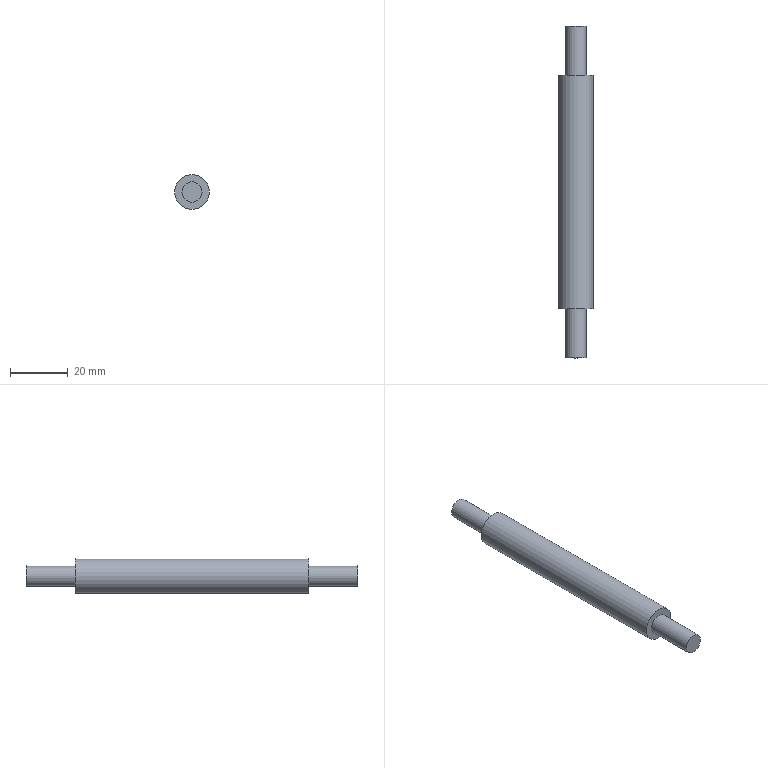Part | STEP file | 2-04.2 | 1 solid | 7 faces | box 12 x 115 x 12 mm | volume 10469 mm3 | plane 4 | cylinder 3 | commonest cylinder face diameters 7 x2 12 x1
STEP:
#1=CARTESIAN_POINT('',(0.,0.,0.));
#2=DIRECTION('',(0.,0.,1.));
#3=DIRECTION('',(1.,0.,0.));
#4=AXIS2_PLACEMENT_3D('',#1,#2,#3);
#5=CARTESIAN_POINT('',(6.,-40.5,0.));
#6=VERTEX_POINT('',#5);
#7=CARTESIAN_POINT('',(6.,40.5,0.));
#8=VERTEX_POINT('',#7);
#9=CARTESIAN_POINT('',(6.,-40.5,0.));
#10=DIRECTION('',(0.,1.,0.));
#11=VECTOR('',#10,1.);
#12=LINE('',#9,#11);
#13=CARTESIAN_POINT('',(0.,-40.5,0.));
#14=DIRECTION('',(0.,1.,0.));
#15=DIRECTION('',(1.,0.,0.));
#16=AXIS2_PLACEMENT_3D('',#13,#14,#15);
#17=CYLINDRICAL_SURFACE('',#16,6.);
#18=CARTESIAN_POINT('',(6.283,0.));
#19=DIRECTION('',(0.,1.));
#20=VECTOR('',#19,1.);
#21=LINE('',#18,#20);
#22=(GEOMETRIC_REPRESENTATION_CONTEXT(2)PARAMETRIC_REPRESENTATION_CONTEXT()REPRESENTATION_CONTEXT('',''));
#23=DEFINITIONAL_REPRESENTATION('',(#21),#22);
#24=PCURVE('',#17,#23);
#25=CARTESIAN_POINT('',(0.,0.));
#26=DIRECTION('',(0.,1.));
#27=VECTOR('',#26,1.);
#28=LINE('',#25,#27);
#29=(GEOMETRIC_REPRESENTATION_CONTEXT(2)PARAMETRIC_REPRESENTATION_CONTEXT()REPRESENTATION_CONTEXT('',''));
#30=DEFINITIONAL_REPRESENTATION('',(#28),#29);
#31=PCURVE('',#17,#30);
#32=SEAM_CURVE('',#12,(#24,#31),.PCURVE_S1.);
#33=EDGE_CURVE('',#6,#8,#32,.T.);
#34=ORIENTED_EDGE('',*,*,#33,.T.);
#35=CARTESIAN_POINT('',(0.,40.5,0.));
#36=DIRECTION('',(0.,-1.,0.));
#37=DIRECTION('',(1.,0.,0.));
#38=AXIS2_PLACEMENT_3D('',#35,#36,#37);
#39=CIRCLE('',#38,6.);
#40=CARTESIAN_POINT('',(6.283,81.));
#41=DIRECTION('',(-1.,0.));
#42=VECTOR('',#41,1.);
#43=LINE('',#40,#42);
#44=(GEOMETRIC_REPRESENTATION_CONTEXT(2)PARAMETRIC_REPRESENTATION_CONTEXT()REPRESENTATION_CONTEXT('',''));
#45=DEFINITIONAL_REPRESENTATION('',(#43),#44);
#46=PCURVE('',#17,#45);
#47=CARTESIAN_POINT('',(-1.608,40.5,0.));
#48=DIRECTION('',(0.,-1.,0.));
#49=DIRECTION('',(1.,0.,0.));
#50=AXIS2_PLACEMENT_3D('',#47,#48,#49);
#51=PLANE('',#50);
#52=CARTESIAN_POINT('',(1.608,0.));
#53=DIRECTION('',(1.,0.));
#54=AXIS2_PLACEMENT_2D('',#52,#53);
#55=CIRCLE('',#54,6.);
#56=(GEOMETRIC_REPRESENTATION_CONTEXT(2)PARAMETRIC_REPRESENTATION_CONTEXT()REPRESENTATION_CONTEXT('',''));
#57=DEFINITIONAL_REPRESENTATION('',(#55),#56);
#58=PCURVE('',#51,#57);
#59=SURFACE_CURVE('',#39,(#46,#58),.PCURVE_S1.);
#60=EDGE_CURVE('',#8,#8,#59,.T.);
#61=ORIENTED_EDGE('',*,*,#60,.T.);
#62=ORIENTED_EDGE('',*,*,#33,.F.);
#63=CARTESIAN_POINT('',(0.,-40.5,0.));
#64=DIRECTION('',(0.,-1.,0.));
#65=DIRECTION('',(1.,0.,0.));
#66=AXIS2_PLACEMENT_3D('',#63,#64,#65);
#67=CIRCLE('',#66,6.);
#68=CARTESIAN_POINT('',(6.283,0.));
#69=DIRECTION('',(-1.,0.));
#70=VECTOR('',#69,1.);
#71=LINE('',#68,#70);
#72=(GEOMETRIC_REPRESENTATION_CONTEXT(2)PARAMETRIC_REPRESENTATION_CONTEXT()REPRESENTATION_CONTEXT('',''));
#73=DEFINITIONAL_REPRESENTATION('',(#71),#72);
#74=PCURVE('',#17,#73);
#75=CARTESIAN_POINT('',(-1.608,-40.5,0.));
#76=DIRECTION('',(0.,-1.,0.));
#77=DIRECTION('',(1.,0.,0.));
#78=AXIS2_PLACEMENT_3D('',#75,#76,#77);
#79=PLANE('',#78);
#80=CARTESIAN_POINT('',(1.608,0.));
#81=DIRECTION('',(1.,0.));
#82=AXIS2_PLACEMENT_2D('',#80,#81);
#83=CIRCLE('',#82,6.);
#84=(GEOMETRIC_REPRESENTATION_CONTEXT(2)PARAMETRIC_REPRESENTATION_CONTEXT()REPRESENTATION_CONTEXT('',''));
#85=DEFINITIONAL_REPRESENTATION('',(#83),#84);
#86=PCURVE('',#79,#85);
#87=SURFACE_CURVE('',#67,(#74,#86),.PCURVE_S1.);
#88=EDGE_CURVE('',#6,#6,#87,.T.);
#89=ORIENTED_EDGE('',*,*,#88,.F.);
#90=EDGE_LOOP('',(#34,#61,#62,#89));
#91=FACE_BOUND('',#90,.T.);
#92=ADVANCED_FACE('',(#91),#17,.T.);
#93=ORIENTED_EDGE('',*,*,#88,.T.);
#94=EDGE_LOOP('',(#93));
#95=FACE_BOUND('',#94,.T.);
#96=CARTESIAN_POINT('',(3.5,-40.5,0.));
#97=VERTEX_POINT('',#96);
#98=CARTESIAN_POINT('',(0.,-40.5,0.));
#99=DIRECTION('',(0.,-1.,0.));
#100=DIRECTION('',(1.,0.,0.));
#101=AXIS2_PLACEMENT_3D('',#98,#99,#100);
#102=CIRCLE('',#101,3.5);
#103=CARTESIAN_POINT('',(1.608,0.));
#104=DIRECTION('',(1.,0.));
#105=AXIS2_PLACEMENT_2D('',#103,#104);
#106=CIRCLE('',#105,3.5);
#107=(GEOMETRIC_REPRESENTATION_CONTEXT(2)PARAMETRIC_REPRESENTATION_CONTEXT()REPRESENTATION_CONTEXT('',''));
#108=DEFINITIONAL_REPRESENTATION('',(#106),#107);
#109=PCURVE('',#79,#108);
#110=CARTESIAN_POINT('',(0.,-40.5,0.));
#111=DIRECTION('',(0.,-1.,0.));
#112=DIRECTION('',(1.,0.,0.));
#113=AXIS2_PLACEMENT_3D('',#110,#111,#112);
#114=CYLINDRICAL_SURFACE('',#113,3.5);
#115=CARTESIAN_POINT('',(0.,0.));
#116=DIRECTION('',(1.,0.));
#117=VECTOR('',#116,1.);
#118=LINE('',#115,#117);
#119=(GEOMETRIC_REPRESENTATION_CONTEXT(2)PARAMETRIC_REPRESENTATION_CONTEXT()REPRESENTATION_CONTEXT('',''));
#120=DEFINITIONAL_REPRESENTATION('',(#118),#119);
#121=PCURVE('',#114,#120);
#122=SURFACE_CURVE('',#102,(#109,#121),.PCURVE_S1.);
#123=EDGE_CURVE('',#97,#97,#122,.T.);
#124=ORIENTED_EDGE('',*,*,#123,.F.);
#125=EDGE_LOOP('',(#124));
#126=FACE_BOUND('',#125,.T.);
#127=ADVANCED_FACE('',(#95,#126),#79,.T.);
#128=ORIENTED_EDGE('',*,*,#123,.T.);
#129=CARTESIAN_POINT('',(3.5,-57.5,0.));
#130=VERTEX_POINT('',#129);
#131=CARTESIAN_POINT('',(3.5,-40.5,0.));
#132=DIRECTION('',(0.,-1.,0.));
#133=VECTOR('',#132,1.);
#134=LINE('',#131,#133);
#135=CARTESIAN_POINT('',(6.283,0.));
#136=DIRECTION('',(0.,1.));
#137=VECTOR('',#136,1.);
#138=LINE('',#135,#137);
#139=(GEOMETRIC_REPRESENTATION_CONTEXT(2)PARAMETRIC_REPRESENTATION_CONTEXT()REPRESENTATION_CONTEXT('',''));
#140=DEFINITIONAL_REPRESENTATION('',(#138),#139);
#141=PCURVE('',#114,#140);
#142=CARTESIAN_POINT('',(0.,0.));
#143=DIRECTION('',(0.,1.));
#144=VECTOR('',#143,1.);
#145=LINE('',#142,#144);
#146=(GEOMETRIC_REPRESENTATION_CONTEXT(2)PARAMETRIC_REPRESENTATION_CONTEXT()REPRESENTATION_CONTEXT('',''));
#147=DEFINITIONAL_REPRESENTATION('',(#145),#146);
#148=PCURVE('',#114,#147);
#149=SEAM_CURVE('',#134,(#141,#148),.PCURVE_S1.);
#150=EDGE_CURVE('',#97,#130,#149,.T.);
#151=ORIENTED_EDGE('',*,*,#150,.T.);
#152=CARTESIAN_POINT('',(0.,-57.5,0.));
#153=DIRECTION('',(0.,-1.,0.));
#154=DIRECTION('',(1.,0.,0.));
#155=AXIS2_PLACEMENT_3D('',#152,#153,#154);
#156=CIRCLE('',#155,3.5);
#157=CARTESIAN_POINT('',(0.,17.));
#158=DIRECTION('',(1.,0.));
#159=VECTOR('',#158,1.);
#160=LINE('',#157,#159);
#161=(GEOMETRIC_REPRESENTATION_CONTEXT(2)PARAMETRIC_REPRESENTATION_CONTEXT()REPRESENTATION_CONTEXT('',''));
#162=DEFINITIONAL_REPRESENTATION('',(#160),#161);
#163=PCURVE('',#114,#162);
#164=CARTESIAN_POINT('',(-0.9378,-57.5,0.));
#165=DIRECTION('',(0.,-1.,0.));
#166=DIRECTION('',(1.,0.,0.));
#167=AXIS2_PLACEMENT_3D('',#164,#165,#166);
#168=PLANE('',#167);
#169=CARTESIAN_POINT('',(0.9378,0.));
#170=DIRECTION('',(1.,0.));
#171=AXIS2_PLACEMENT_2D('',#169,#170);
#172=CIRCLE('',#171,3.5);
#173=(GEOMETRIC_REPRESENTATION_CONTEXT(2)PARAMETRIC_REPRESENTATION_CONTEXT()REPRESENTATION_CONTEXT('',''));
#174=DEFINITIONAL_REPRESENTATION('',(#172),#173);
#175=PCURVE('',#168,#174);
#176=SURFACE_CURVE('',#156,(#163,#175),.PCURVE_S1.);
#177=EDGE_CURVE('',#130,#130,#176,.T.);
#178=ORIENTED_EDGE('',*,*,#177,.F.);
#179=ORIENTED_EDGE('',*,*,#150,.F.);
#180=EDGE_LOOP('',(#128,#151,#178,#179));
#181=FACE_BOUND('',#180,.T.);
#182=ADVANCED_FACE('',(#181),#114,.T.);
#183=ORIENTED_EDGE('',*,*,#177,.T.);
#184=EDGE_LOOP('',(#183));
#185=FACE_BOUND('',#184,.T.);
#186=ADVANCED_FACE('',(#185),#168,.T.);
#187=ORIENTED_EDGE('',*,*,#60,.T.);
#188=EDGE_LOOP('',(#187));
#189=FACE_BOUND('',#188,.F.);
#190=CARTESIAN_POINT('',(3.5,40.5,0.));
#191=VERTEX_POINT('',#190);
#192=CARTESIAN_POINT('',(0.,40.5,0.));
#193=DIRECTION('',(0.,-1.,0.));
#194=DIRECTION('',(1.,0.,0.));
#195=AXIS2_PLACEMENT_3D('',#192,#193,#194);
#196=CIRCLE('',#195,3.5);
#197=CARTESIAN_POINT('',(1.608,0.));
#198=DIRECTION('',(1.,0.));
#199=AXIS2_PLACEMENT_2D('',#197,#198);
#200=CIRCLE('',#199,3.5);
#201=(GEOMETRIC_REPRESENTATION_CONTEXT(2)PARAMETRIC_REPRESENTATION_CONTEXT()REPRESENTATION_CONTEXT('',''));
#202=DEFINITIONAL_REPRESENTATION('',(#200),#201);
#203=PCURVE('',#51,#202);
#204=CARTESIAN_POINT('',(0.,40.5,0.));
#205=DIRECTION('',(0.,1.,0.));
#206=DIRECTION('',(1.,0.,0.));
#207=AXIS2_PLACEMENT_3D('',#204,#205,#206);
#208=CYLINDRICAL_SURFACE('',#207,3.5);
#209=CARTESIAN_POINT('',(6.283,0.));
#210=DIRECTION('',(-1.,0.));
#211=VECTOR('',#210,1.);
#212=LINE('',#209,#211);
#213=(GEOMETRIC_REPRESENTATION_CONTEXT(2)PARAMETRIC_REPRESENTATION_CONTEXT()REPRESENTATION_CONTEXT('',''));
#214=DEFINITIONAL_REPRESENTATION('',(#212),#213);
#215=PCURVE('',#208,#214);
#216=SURFACE_CURVE('',#196,(#203,#215),.PCURVE_S1.);
#217=EDGE_CURVE('',#191,#191,#216,.T.);
#218=ORIENTED_EDGE('',*,*,#217,.F.);
#219=EDGE_LOOP('',(#218));
#220=FACE_BOUND('',#219,.F.);
#221=ADVANCED_FACE('',(#189,#220),#51,.F.);
#222=CARTESIAN_POINT('',(3.5,57.5,0.));
#223=VERTEX_POINT('',#222);
#224=CARTESIAN_POINT('',(3.5,40.5,0.));
#225=DIRECTION('',(0.,1.,0.));
#226=VECTOR('',#225,1.);
#227=LINE('',#224,#226);
#228=CARTESIAN_POINT('',(6.283,0.));
#229=DIRECTION('',(0.,1.));
#230=VECTOR('',#229,1.);
#231=LINE('',#228,#230);
#232=(GEOMETRIC_REPRESENTATION_CONTEXT(2)PARAMETRIC_REPRESENTATION_CONTEXT()REPRESENTATION_CONTEXT('',''));
#233=DEFINITIONAL_REPRESENTATION('',(#231),#232);
#234=PCURVE('',#208,#233);
#235=CARTESIAN_POINT('',(0.,0.));
#236=DIRECTION('',(0.,1.));
#237=VECTOR('',#236,1.);
#238=LINE('',#235,#237);
#239=(GEOMETRIC_REPRESENTATION_CONTEXT(2)PARAMETRIC_REPRESENTATION_CONTEXT()REPRESENTATION_CONTEXT('',''));
#240=DEFINITIONAL_REPRESENTATION('',(#238),#239);
#241=PCURVE('',#208,#240);
#242=SEAM_CURVE('',#227,(#234,#241),.PCURVE_S1.);
#243=EDGE_CURVE('',#191,#223,#242,.T.);
#244=ORIENTED_EDGE('',*,*,#243,.T.);
#245=CARTESIAN_POINT('',(0.,57.5,0.));
#246=DIRECTION('',(0.,-1.,0.));
#247=DIRECTION('',(1.,0.,0.));
#248=AXIS2_PLACEMENT_3D('',#245,#246,#247);
#249=CIRCLE('',#248,3.5);
#250=CARTESIAN_POINT('',(6.283,17.));
#251=DIRECTION('',(-1.,0.));
#252=VECTOR('',#251,1.);
#253=LINE('',#250,#252);
#254=(GEOMETRIC_REPRESENTATION_CONTEXT(2)PARAMETRIC_REPRESENTATION_CONTEXT()REPRESENTATION_CONTEXT('',''));
#255=DEFINITIONAL_REPRESENTATION('',(#253),#254);
#256=PCURVE('',#208,#255);
#257=CARTESIAN_POINT('',(-0.9378,57.5,0.));
#258=DIRECTION('',(0.,-1.,0.));
#259=DIRECTION('',(1.,0.,0.));
#260=AXIS2_PLACEMENT_3D('',#257,#258,#259);
#261=PLANE('',#260);
#262=CARTESIAN_POINT('',(0.9378,0.));
#263=DIRECTION('',(1.,0.));
#264=AXIS2_PLACEMENT_2D('',#262,#263);
#265=CIRCLE('',#264,3.5);
#266=(GEOMETRIC_REPRESENTATION_CONTEXT(2)PARAMETRIC_REPRESENTATION_CONTEXT()REPRESENTATION_CONTEXT('',''));
#267=DEFINITIONAL_REPRESENTATION('',(#265),#266);
#268=PCURVE('',#261,#267);
#269=SURFACE_CURVE('',#249,(#256,#268),.PCURVE_S1.);
#270=EDGE_CURVE('',#223,#223,#269,.T.);
#271=ORIENTED_EDGE('',*,*,#270,.T.);
#272=ORIENTED_EDGE('',*,*,#243,.F.);
#273=ORIENTED_EDGE('',*,*,#217,.F.);
#274=EDGE_LOOP('',(#244,#271,#272,#273));
#275=FACE_BOUND('',#274,.T.);
#276=ADVANCED_FACE('',(#275),#208,.T.);
#277=ORIENTED_EDGE('',*,*,#270,.T.);
#278=EDGE_LOOP('',(#277));
#279=FACE_BOUND('',#278,.F.);
#280=ADVANCED_FACE('',(#279),#261,.F.);
#281=CLOSED_SHELL('',(#92,#127,#182,#186,#221,#276,#280));
#282=MANIFOLD_SOLID_BREP('',#281);
#283=(LENGTH_UNIT()NAMED_UNIT(*)SI_UNIT(.MILLI.,.METRE.));
#284=UNCERTAINTY_MEASURE_WITH_UNIT(LENGTH_MEASURE(0.0000001),#283,'','');
#285=(NAMED_UNIT(*)PLANE_ANGLE_UNIT()SI_UNIT($,.RADIAN.));
#286=(NAMED_UNIT(*)SI_UNIT($,.STERADIAN.)SOLID_ANGLE_UNIT());
#287=(GEOMETRIC_REPRESENTATION_CONTEXT(3)GLOBAL_UNCERTAINTY_ASSIGNED_CONTEXT((#284))GLOBAL_UNIT_ASSIGNED_CONTEXT((#283,#285,#286))REPRESENTATION_CONTEXT('',''));
#288=ADVANCED_BREP_SHAPE_REPRESENTATION('',(#4,#282),#287);